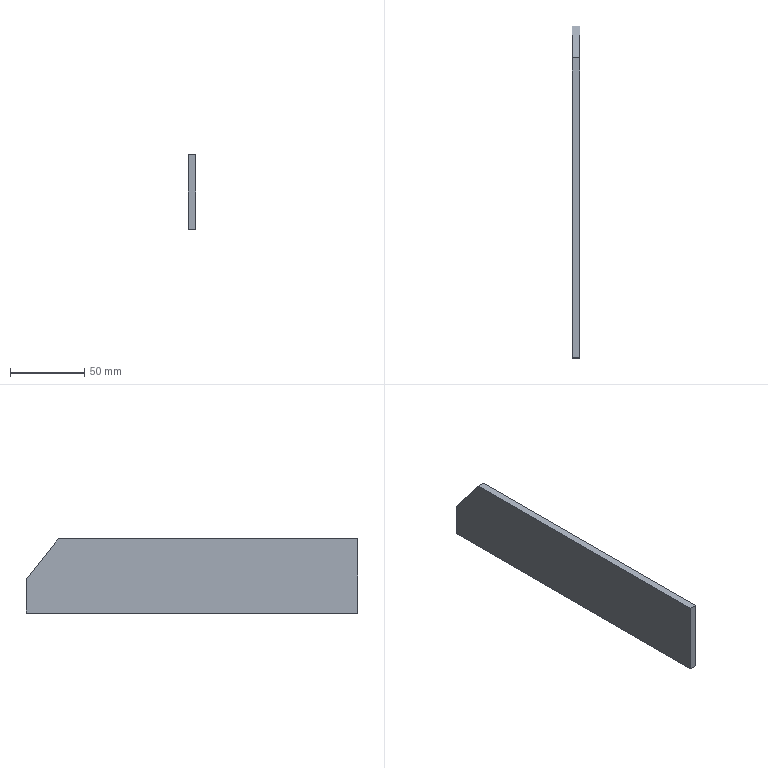Part | SolidWorks | features BaseBody 1 | 1 solid | 7 faces | box 5 x 224.044 x 50.002 mm | volume 54532 mm3 | plane 7
STEP:
#1=CARTESIAN_POINT('',(244.446,-4144.517,1052.974));
#2=VERTEX_POINT('',#1);
#3=CARTESIAN_POINT('',(244.446,-3942.094,1052.974));
#4=VERTEX_POINT('',#3);
#5=CARTESIAN_POINT('',(244.446,-4035.726,1052.974));
#6=DIRECTION('',(0.,1.,0.));
#7=VECTOR('',#6,1000.);
#8=LINE('',#5,#7);
#9=EDGE_CURVE('',#2,#4,#8,.T.);
#10=ORIENTED_EDGE('',*,*,#9,.F.);
#11=CARTESIAN_POINT('',(244.446,-4144.517,1002.971));
#12=VERTEX_POINT('',#11);
#13=CARTESIAN_POINT('',(244.446,-4144.517,1027.093));
#14=DIRECTION('',(0.,0.,1.));
#15=VECTOR('',#14,1000.);
#16=LINE('',#13,#15);
#17=EDGE_CURVE('',#12,#2,#16,.T.);
#18=ORIENTED_EDGE('',*,*,#17,.F.);
#19=CARTESIAN_POINT('',(244.446,-3920.473,1002.971));
#20=VERTEX_POINT('',#19);
#21=CARTESIAN_POINT('',(244.446,-4035.726,1002.971));
#22=DIRECTION('',(0.,-1.,0.));
#23=VECTOR('',#22,1000.);
#24=LINE('',#21,#23);
#25=EDGE_CURVE('',#20,#12,#24,.T.);
#26=ORIENTED_EDGE('',*,*,#25,.F.);
#27=CARTESIAN_POINT('',(244.446,-3920.473,1025.564));
#28=VERTEX_POINT('',#27);
#29=CARTESIAN_POINT('',(244.446,-3920.473,1027.093));
#30=DIRECTION('',(0.,0.,-1.));
#31=VECTOR('',#30,1000.);
#32=LINE('',#29,#31);
#33=EDGE_CURVE('',#28,#20,#32,.T.);
#34=ORIENTED_EDGE('',*,*,#33,.F.);
#35=CARTESIAN_POINT('',(244.446,-3942.094,1052.974));
#36=DIRECTION('',(0.,0.6193,-0.7851));
#37=VECTOR('',#36,1000.);
#38=LINE('',#35,#37);
#39=EDGE_CURVE('',#4,#28,#38,.T.);
#40=ORIENTED_EDGE('',*,*,#39,.F.);
#41=EDGE_LOOP('',(#10,#18,#26,#34,#40));
#42=FACE_OUTER_BOUND('',#41,.T.);
#43=CARTESIAN_POINT('',(244.446,-4035.726,1027.093));
#44=DIRECTION('',(-1.,0.,0.));
#45=DIRECTION('',(0.,0.,1.));
#46=AXIS2_PLACEMENT_3D('',#43,#44,#45);
#47=PLANE('',#46);
#48=ADVANCED_FACE('',(#42),#47,.F.);
#49=ORIENTED_EDGE('',*,*,#39,.T.);
#50=CARTESIAN_POINT('',(239.446,-3920.473,1025.564));
#51=VERTEX_POINT('',#50);
#52=CARTESIAN_POINT('',(244.446,-3920.473,1025.564));
#53=DIRECTION('',(-1.,0.,0.));
#54=VECTOR('',#53,1000.);
#55=LINE('',#52,#54);
#56=EDGE_CURVE('',#28,#51,#55,.T.);
#57=ORIENTED_EDGE('',*,*,#56,.T.);
#58=CARTESIAN_POINT('',(239.446,-3942.094,1052.974));
#59=VERTEX_POINT('',#58);
#60=CARTESIAN_POINT('',(239.446,-3920.473,1025.564));
#61=DIRECTION('',(0.,-0.6193,0.7851));
#62=VECTOR('',#61,1000.);
#63=LINE('',#60,#62);
#64=EDGE_CURVE('',#51,#59,#63,.T.);
#65=ORIENTED_EDGE('',*,*,#64,.T.);
#66=CARTESIAN_POINT('',(244.446,-3942.094,1052.974));
#67=DIRECTION('',(1.,0.,0.));
#68=VECTOR('',#67,1000.);
#69=LINE('',#66,#68);
#70=EDGE_CURVE('',#59,#4,#69,.T.);
#71=ORIENTED_EDGE('',*,*,#70,.T.);
#72=EDGE_LOOP('',(#49,#57,#65,#71));
#73=FACE_OUTER_BOUND('',#72,.T.);
#74=CARTESIAN_POINT('',(244.446,-3920.473,1025.564));
#75=DIRECTION('',(0.,0.7851,0.6193));
#76=DIRECTION('',(0.,-0.6193,0.7851));
#77=AXIS2_PLACEMENT_3D('',#74,#75,#76);
#78=PLANE('',#77);
#79=ADVANCED_FACE('',(#73),#78,.T.);
#80=ORIENTED_EDGE('',*,*,#9,.T.);
#81=ORIENTED_EDGE('',*,*,#70,.F.);
#82=CARTESIAN_POINT('',(239.446,-4144.517,1052.974));
#83=VERTEX_POINT('',#82);
#84=CARTESIAN_POINT('',(239.446,-3942.094,1052.974));
#85=DIRECTION('',(0.,-1.,0.));
#86=VECTOR('',#85,1000.);
#87=LINE('',#84,#86);
#88=EDGE_CURVE('',#59,#83,#87,.T.);
#89=ORIENTED_EDGE('',*,*,#88,.T.);
#90=CARTESIAN_POINT('',(244.446,-4144.517,1052.974));
#91=DIRECTION('',(1.,0.,0.));
#92=VECTOR('',#91,1000.);
#93=LINE('',#90,#92);
#94=EDGE_CURVE('',#83,#2,#93,.T.);
#95=ORIENTED_EDGE('',*,*,#94,.T.);
#96=EDGE_LOOP('',(#80,#81,#89,#95));
#97=FACE_OUTER_BOUND('',#96,.T.);
#98=CARTESIAN_POINT('',(244.446,-3942.094,1052.974));
#99=DIRECTION('',(0.,0.,1.));
#100=DIRECTION('',(1.,0.,0.));
#101=AXIS2_PLACEMENT_3D('',#98,#99,#100);
#102=PLANE('',#101);
#103=ADVANCED_FACE('',(#97),#102,.T.);
#104=ORIENTED_EDGE('',*,*,#17,.T.);
#105=ORIENTED_EDGE('',*,*,#94,.F.);
#106=CARTESIAN_POINT('',(239.446,-4144.517,1002.971));
#107=VERTEX_POINT('',#106);
#108=CARTESIAN_POINT('',(239.446,-4144.517,1052.974));
#109=DIRECTION('',(0.,0.,-1.));
#110=VECTOR('',#109,1000.);
#111=LINE('',#108,#110);
#112=EDGE_CURVE('',#83,#107,#111,.T.);
#113=ORIENTED_EDGE('',*,*,#112,.T.);
#114=CARTESIAN_POINT('',(244.446,-4144.517,1002.971));
#115=DIRECTION('',(1.,0.,0.));
#116=VECTOR('',#115,1000.);
#117=LINE('',#114,#116);
#118=EDGE_CURVE('',#107,#12,#117,.T.);
#119=ORIENTED_EDGE('',*,*,#118,.T.);
#120=EDGE_LOOP('',(#104,#105,#113,#119));
#121=FACE_OUTER_BOUND('',#120,.T.);
#122=CARTESIAN_POINT('',(244.446,-4144.517,1052.974));
#123=DIRECTION('',(0.,-1.,0.));
#124=DIRECTION('',(0.,0.,-1.));
#125=AXIS2_PLACEMENT_3D('',#122,#123,#124);
#126=PLANE('',#125);
#127=ADVANCED_FACE('',(#121),#126,.T.);
#128=ORIENTED_EDGE('',*,*,#25,.T.);
#129=ORIENTED_EDGE('',*,*,#118,.F.);
#130=CARTESIAN_POINT('',(239.446,-3920.473,1002.971));
#131=VERTEX_POINT('',#130);
#132=CARTESIAN_POINT('',(239.446,-4144.517,1002.971));
#133=DIRECTION('',(0.,1.,0.));
#134=VECTOR('',#133,1000.);
#135=LINE('',#132,#134);
#136=EDGE_CURVE('',#107,#131,#135,.T.);
#137=ORIENTED_EDGE('',*,*,#136,.T.);
#138=CARTESIAN_POINT('',(244.446,-3920.473,1002.971));
#139=DIRECTION('',(1.,0.,0.));
#140=VECTOR('',#139,1000.);
#141=LINE('',#138,#140);
#142=EDGE_CURVE('',#131,#20,#141,.T.);
#143=ORIENTED_EDGE('',*,*,#142,.T.);
#144=EDGE_LOOP('',(#128,#129,#137,#143));
#145=FACE_OUTER_BOUND('',#144,.T.);
#146=CARTESIAN_POINT('',(244.446,-4144.517,1002.971));
#147=DIRECTION('',(0.,0.,-1.));
#148=DIRECTION('',(-1.,0.,0.));
#149=AXIS2_PLACEMENT_3D('',#146,#147,#148);
#150=PLANE('',#149);
#151=ADVANCED_FACE('',(#145),#150,.T.);
#152=ORIENTED_EDGE('',*,*,#33,.T.);
#153=ORIENTED_EDGE('',*,*,#142,.F.);
#154=CARTESIAN_POINT('',(239.446,-3920.473,1002.921));
#155=DIRECTION('',(0.,0.,1.));
#156=VECTOR('',#155,1000.);
#157=LINE('',#154,#156);
#158=EDGE_CURVE('',#131,#51,#157,.T.);
#159=ORIENTED_EDGE('',*,*,#158,.T.);
#160=ORIENTED_EDGE('',*,*,#56,.F.);
#161=EDGE_LOOP('',(#152,#153,#159,#160));
#162=FACE_OUTER_BOUND('',#161,.T.);
#163=CARTESIAN_POINT('',(244.446,-3920.473,1002.921));
#164=DIRECTION('',(0.,1.,0.));
#165=DIRECTION('',(0.,0.,1.));
#166=AXIS2_PLACEMENT_3D('',#163,#164,#165);
#167=PLANE('',#166);
#168=ADVANCED_FACE('',(#162),#167,.T.);
#169=ORIENTED_EDGE('',*,*,#136,.F.);
#170=ORIENTED_EDGE('',*,*,#112,.F.);
#171=ORIENTED_EDGE('',*,*,#88,.F.);
#172=ORIENTED_EDGE('',*,*,#64,.F.);
#173=ORIENTED_EDGE('',*,*,#158,.F.);
#174=EDGE_LOOP('',(#169,#170,#171,#172,#173));
#175=FACE_OUTER_BOUND('',#174,.T.);
#176=CARTESIAN_POINT('',(239.446,-4035.726,1027.143));
#177=DIRECTION('',(-1.,0.,0.));
#178=DIRECTION('',(0.,0.,1.));
#179=AXIS2_PLACEMENT_3D('',#176,#177,#178);
#180=PLANE('',#179);
#181=ADVANCED_FACE('',(#175),#180,.T.);
#182=CLOSED_SHELL('',(#48,#79,#103,#127,#151,#168,#181));
#183=MANIFOLD_SOLID_BREP('',#182);
#184=CARTESIAN_POINT('',(0.,0.,0.));
#185=DIRECTION('',(0.,0.,1.));
#186=DIRECTION('',(1.,0.,0.));
#187=AXIS2_PLACEMENT_3D('',#184,#185,#186);
#188=(LENGTH_UNIT()NAMED_UNIT(*)SI_UNIT(.MILLI.,.METRE.));
#189=UNCERTAINTY_MEASURE_WITH_UNIT(LENGTH_MEASURE(0.00001),#188,'','');
#190=(NAMED_UNIT(*)PLANE_ANGLE_UNIT()SI_UNIT($,.RADIAN.));
#191=(NAMED_UNIT(*)SI_UNIT($,.STERADIAN.)SOLID_ANGLE_UNIT());
#192=(GEOMETRIC_REPRESENTATION_CONTEXT(3)GLOBAL_UNCERTAINTY_ASSIGNED_CONTEXT((#189))GLOBAL_UNIT_ASSIGNED_CONTEXT((#188,#190,#191))REPRESENTATION_CONTEXT('',''));
#193=ADVANCED_BREP_SHAPE_REPRESENTATION('',(#183,#187),#192);